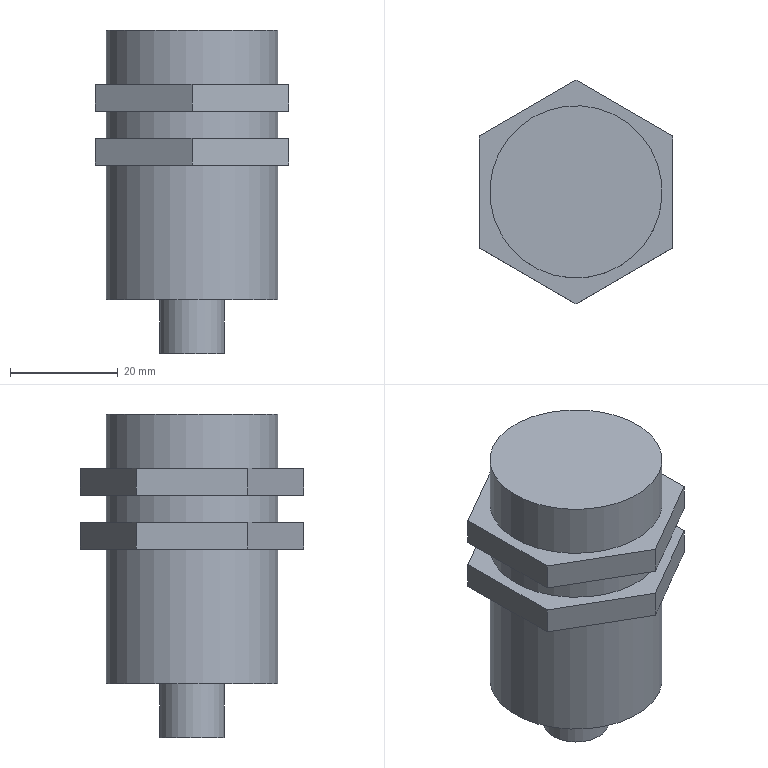Part | NX | features solid 2 | 1 solid | 23 faces | box 36 x 41.569 x 60 mm | volume 44525 mm3 | plane 19 | cylinder 4 | commonest cylinder face diameters 32 x3 12 x1
STEP:
#1=CARTESIAN_POINT('',(1648.644,144.279,-60.));
#2=VERTEX_POINT('',#1);
#3=CARTESIAN_POINT('',(1634.788,136.279,-60.));
#4=DIRECTION('',(0.,0.,-1.));
#5=DIRECTION('',(0.866,0.5,0.));
#6=AXIS2_PLACEMENT_3D('',#3,#4,#5);
#7=CIRCLE('',#6,16.);
#8=EDGE_CURVE('',#2,#2,#7,.T.);
#9=ORIENTED_EDGE('',*,*,#8,.F.);
#10=EDGE_LOOP('',(#9));
#11=FACE_BOUND('',#10,.T.);
#12=CARTESIAN_POINT('',(1648.644,144.279,-55.));
#13=VERTEX_POINT('',#12);
#14=CARTESIAN_POINT('',(1634.788,136.279,-55.));
#15=DIRECTION('',(0.,0.,-1.));
#16=DIRECTION('',(0.866,0.5,0.));
#17=AXIS2_PLACEMENT_3D('',#14,#15,#16);
#18=CIRCLE('',#17,16.);
#19=EDGE_CURVE('',#13,#13,#18,.T.);
#20=ORIENTED_EDGE('',*,*,#19,.T.);
#21=EDGE_LOOP('',(#20));
#22=FACE_BOUND('',#21,.T.);
#23=CARTESIAN_POINT('',(1634.788,136.279,-40.));
#24=DIRECTION('',(0.,0.,-1.));
#25=DIRECTION('',(-0.866,-0.5,0.));
#26=AXIS2_PLACEMENT_3D('',#23,#24,#25);
#27=CYLINDRICAL_SURFACE('',#26,16.);
#28=ADVANCED_FACE('',(#11,#22),#27,.T.);
#29=CARTESIAN_POINT('',(1648.644,144.279,-90.));
#30=VERTEX_POINT('',#29);
#31=CARTESIAN_POINT('',(1634.788,136.279,-90.));
#32=DIRECTION('',(0.,0.,-1.));
#33=DIRECTION('',(0.866,0.5,0.));
#34=AXIS2_PLACEMENT_3D('',#31,#32,#33);
#35=CIRCLE('',#34,16.);
#36=EDGE_CURVE('',#30,#30,#35,.T.);
#37=ORIENTED_EDGE('',*,*,#36,.F.);
#38=EDGE_LOOP('',(#37));
#39=FACE_BOUND('',#38,.T.);
#40=CARTESIAN_POINT('',(1648.644,144.279,-65.));
#41=VERTEX_POINT('',#40);
#42=CARTESIAN_POINT('',(1634.788,136.279,-65.));
#43=DIRECTION('',(0.,0.,-1.));
#44=DIRECTION('',(0.866,0.5,0.));
#45=AXIS2_PLACEMENT_3D('',#42,#43,#44);
#46=CIRCLE('',#45,16.);
#47=EDGE_CURVE('',#41,#41,#46,.T.);
#48=ORIENTED_EDGE('',*,*,#47,.T.);
#49=EDGE_LOOP('',(#48));
#50=FACE_BOUND('',#49,.T.);
#51=CARTESIAN_POINT('',(1634.788,136.279,-40.));
#52=DIRECTION('',(0.,0.,-1.));
#53=DIRECTION('',(-0.866,-0.5,0.));
#54=AXIS2_PLACEMENT_3D('',#51,#52,#53);
#55=CYLINDRICAL_SURFACE('',#54,16.);
#56=ADVANCED_FACE('',(#39,#50),#55,.T.);
#57=CARTESIAN_POINT('',(1639.984,139.279,-90.));
#58=VERTEX_POINT('',#57);
#59=CARTESIAN_POINT('',(1634.788,136.279,-90.));
#60=DIRECTION('',(0.,0.,-1.));
#61=DIRECTION('',(0.866,0.5,0.));
#62=AXIS2_PLACEMENT_3D('',#59,#60,#61);
#63=CIRCLE('',#62,6.);
#64=EDGE_CURVE('',#58,#58,#63,.T.);
#65=ORIENTED_EDGE('',*,*,#64,.T.);
#66=EDGE_LOOP('',(#65));
#67=FACE_BOUND('',#66,.T.);
#68=CARTESIAN_POINT('',(1639.984,139.279,-100.));
#69=VERTEX_POINT('',#68);
#70=CARTESIAN_POINT('',(1634.788,136.279,-100.));
#71=DIRECTION('',(0.,0.,-1.));
#72=DIRECTION('',(0.866,0.5,0.));
#73=AXIS2_PLACEMENT_3D('',#70,#71,#72);
#74=CIRCLE('',#73,6.);
#75=EDGE_CURVE('',#69,#69,#74,.T.);
#76=ORIENTED_EDGE('',*,*,#75,.F.);
#77=EDGE_LOOP('',(#76));
#78=FACE_BOUND('',#77,.T.);
#79=CARTESIAN_POINT('',(1634.788,136.279,-90.));
#80=DIRECTION('',(0.,0.,-1.));
#81=DIRECTION('',(-0.866,-0.5,0.));
#82=AXIS2_PLACEMENT_3D('',#79,#80,#81);
#83=CYLINDRICAL_SURFACE('',#82,6.);
#84=ADVANCED_FACE('',(#67,#78),#83,.T.);
#85=ORIENTED_EDGE('',*,*,#75,.T.);
#86=EDGE_LOOP('',(#85));
#87=FACE_BOUND('',#86,.T.);
#88=CARTESIAN_POINT('',(1634.788,136.279,-100.));
#89=DIRECTION('',(0.,0.,1.));
#90=DIRECTION('',(0.866,0.5,0.));
#91=AXIS2_PLACEMENT_3D('',#88,#89,#90);
#92=PLANE('',#91);
#93=ADVANCED_FACE('',(#87),#92,.F.);
#94=ORIENTED_EDGE('',*,*,#36,.T.);
#95=EDGE_LOOP('',(#94));
#96=FACE_BOUND('',#95,.T.);
#97=ORIENTED_EDGE('',*,*,#64,.F.);
#98=EDGE_LOOP('',(#97));
#99=FACE_BOUND('',#98,.T.);
#100=CARTESIAN_POINT('',(1634.788,136.279,-90.));
#101=DIRECTION('',(0.,0.,1.));
#102=DIRECTION('',(0.866,0.5,0.));
#103=AXIS2_PLACEMENT_3D('',#100,#101,#102);
#104=PLANE('',#103);
#105=ADVANCED_FACE('',(#96,#99),#104,.F.);
#106=CARTESIAN_POINT('',(1616.788,125.887,-60.));
#107=VERTEX_POINT('',#106);
#108=CARTESIAN_POINT('',(1634.788,115.495,-60.));
#109=VERTEX_POINT('',#108);
#110=CARTESIAN_POINT('',(1616.788,125.887,-60.));
#111=DIRECTION('',(0.866,-0.5,0.));
#112=VECTOR('',#111,1000.);
#113=LINE('',#110,#112);
#114=EDGE_CURVE('',#107,#109,#113,.T.);
#115=ORIENTED_EDGE('',*,*,#114,.T.);
#116=CARTESIAN_POINT('',(1652.788,125.887,-60.));
#117=VERTEX_POINT('',#116);
#118=CARTESIAN_POINT('',(1634.788,115.495,-60.));
#119=DIRECTION('',(0.866,0.5,0.));
#120=VECTOR('',#119,1000.);
#121=LINE('',#118,#120);
#122=EDGE_CURVE('',#109,#117,#121,.T.);
#123=ORIENTED_EDGE('',*,*,#122,.T.);
#124=CARTESIAN_POINT('',(1652.788,146.672,-60.));
#125=VERTEX_POINT('',#124);
#126=CARTESIAN_POINT('',(1652.788,146.672,-60.));
#127=DIRECTION('',(0.,-1.,0.));
#128=VECTOR('',#127,1000.);
#129=LINE('',#126,#128);
#130=EDGE_CURVE('',#125,#117,#129,.T.);
#131=ORIENTED_EDGE('',*,*,#130,.F.);
#132=CARTESIAN_POINT('',(1634.788,157.064,-60.));
#133=VERTEX_POINT('',#132);
#134=CARTESIAN_POINT('',(1652.788,146.672,-60.));
#135=DIRECTION('',(-0.866,0.5,0.));
#136=VECTOR('',#135,1000.);
#137=LINE('',#134,#136);
#138=EDGE_CURVE('',#125,#133,#137,.T.);
#139=ORIENTED_EDGE('',*,*,#138,.T.);
#140=CARTESIAN_POINT('',(1616.788,146.672,-60.));
#141=VERTEX_POINT('',#140);
#142=CARTESIAN_POINT('',(1634.788,157.064,-60.));
#143=DIRECTION('',(-0.866,-0.5,0.));
#144=VECTOR('',#143,1000.);
#145=LINE('',#142,#144);
#146=EDGE_CURVE('',#133,#141,#145,.T.);
#147=ORIENTED_EDGE('',*,*,#146,.T.);
#148=CARTESIAN_POINT('',(1616.788,146.672,-60.));
#149=DIRECTION('',(0.,-1.,0.));
#150=VECTOR('',#149,1000.);
#151=LINE('',#148,#150);
#152=EDGE_CURVE('',#141,#107,#151,.T.);
#153=ORIENTED_EDGE('',*,*,#152,.T.);
#154=EDGE_LOOP('',(#115,#123,#131,#139,#147,#153));
#155=FACE_BOUND('',#154,.T.);
#156=ORIENTED_EDGE('',*,*,#8,.T.);
#157=EDGE_LOOP('',(#156));
#158=FACE_BOUND('',#157,.T.);
#159=CARTESIAN_POINT('',(1652.788,105.103,-60.));
#160=DIRECTION('',(0.,0.,1.));
#161=DIRECTION('',(0.866,0.5,0.));
#162=AXIS2_PLACEMENT_3D('',#159,#160,#161);
#163=PLANE('',#162);
#164=ADVANCED_FACE('',(#155,#158),#163,.T.);
#165=CARTESIAN_POINT('',(1616.788,125.887,-65.));
#166=VERTEX_POINT('',#165);
#167=CARTESIAN_POINT('',(1634.788,115.495,-65.));
#168=VERTEX_POINT('',#167);
#169=CARTESIAN_POINT('',(1616.788,125.887,-65.));
#170=DIRECTION('',(0.866,-0.5,0.));
#171=VECTOR('',#170,1000.);
#172=LINE('',#169,#171);
#173=EDGE_CURVE('',#166,#168,#172,.T.);
#174=ORIENTED_EDGE('',*,*,#173,.F.);
#175=CARTESIAN_POINT('',(1616.788,146.672,-65.));
#176=VERTEX_POINT('',#175);
#177=CARTESIAN_POINT('',(1616.788,146.672,-65.));
#178=DIRECTION('',(0.,-1.,0.));
#179=VECTOR('',#178,1000.);
#180=LINE('',#177,#179);
#181=EDGE_CURVE('',#176,#166,#180,.T.);
#182=ORIENTED_EDGE('',*,*,#181,.F.);
#183=CARTESIAN_POINT('',(1634.788,157.064,-65.));
#184=VERTEX_POINT('',#183);
#185=CARTESIAN_POINT('',(1634.788,157.064,-65.));
#186=DIRECTION('',(-0.866,-0.5,0.));
#187=VECTOR('',#186,1000.);
#188=LINE('',#185,#187);
#189=EDGE_CURVE('',#184,#176,#188,.T.);
#190=ORIENTED_EDGE('',*,*,#189,.F.);
#191=CARTESIAN_POINT('',(1652.788,146.672,-65.));
#192=VERTEX_POINT('',#191);
#193=CARTESIAN_POINT('',(1652.788,146.672,-65.));
#194=DIRECTION('',(-0.866,0.5,0.));
#195=VECTOR('',#194,1000.);
#196=LINE('',#193,#195);
#197=EDGE_CURVE('',#192,#184,#196,.T.);
#198=ORIENTED_EDGE('',*,*,#197,.F.);
#199=CARTESIAN_POINT('',(1652.788,125.887,-65.));
#200=VERTEX_POINT('',#199);
#201=CARTESIAN_POINT('',(1652.788,146.672,-65.));
#202=DIRECTION('',(0.,-1.,0.));
#203=VECTOR('',#202,1000.);
#204=LINE('',#201,#203);
#205=EDGE_CURVE('',#192,#200,#204,.T.);
#206=ORIENTED_EDGE('',*,*,#205,.T.);
#207=CARTESIAN_POINT('',(1634.788,115.495,-65.));
#208=DIRECTION('',(0.866,0.5,0.));
#209=VECTOR('',#208,1000.);
#210=LINE('',#207,#209);
#211=EDGE_CURVE('',#168,#200,#210,.T.);
#212=ORIENTED_EDGE('',*,*,#211,.F.);
#213=EDGE_LOOP('',(#174,#182,#190,#198,#206,#212));
#214=FACE_BOUND('',#213,.T.);
#215=ORIENTED_EDGE('',*,*,#47,.F.);
#216=EDGE_LOOP('',(#215));
#217=FACE_BOUND('',#216,.T.);
#218=CARTESIAN_POINT('',(1652.788,105.103,-65.));
#219=DIRECTION('',(0.,0.,1.));
#220=DIRECTION('',(0.866,0.5,0.));
#221=AXIS2_PLACEMENT_3D('',#218,#219,#220);
#222=PLANE('',#221);
#223=ADVANCED_FACE('',(#214,#217),#222,.F.);
#224=ORIENTED_EDGE('',*,*,#173,.T.);
#225=CARTESIAN_POINT('',(1634.788,115.495,-60.));
#226=DIRECTION('',(0.,0.,-1.));
#227=VECTOR('',#226,1000.);
#228=LINE('',#225,#227);
#229=EDGE_CURVE('',#109,#168,#228,.T.);
#230=ORIENTED_EDGE('',*,*,#229,.F.);
#231=ORIENTED_EDGE('',*,*,#114,.F.);
#232=CARTESIAN_POINT('',(1616.788,125.887,-60.));
#233=DIRECTION('',(0.,0.,-1.));
#234=VECTOR('',#233,1000.);
#235=LINE('',#232,#234);
#236=EDGE_CURVE('',#107,#166,#235,.T.);
#237=ORIENTED_EDGE('',*,*,#236,.T.);
#238=EDGE_LOOP('',(#224,#230,#231,#237));
#239=FACE_BOUND('',#238,.T.);
#240=CARTESIAN_POINT('',(1616.788,125.887,-60.));
#241=DIRECTION('',(-0.5,-0.866,0.));
#242=DIRECTION('',(-0.866,0.5,0.));
#243=AXIS2_PLACEMENT_3D('',#240,#241,#242);
#244=PLANE('',#243);
#245=ADVANCED_FACE('',(#239),#244,.T.);
#246=ORIENTED_EDGE('',*,*,#211,.T.);
#247=CARTESIAN_POINT('',(1652.788,125.887,-60.));
#248=DIRECTION('',(0.,0.,-1.));
#249=VECTOR('',#248,1000.);
#250=LINE('',#247,#249);
#251=EDGE_CURVE('',#117,#200,#250,.T.);
#252=ORIENTED_EDGE('',*,*,#251,.F.);
#253=ORIENTED_EDGE('',*,*,#122,.F.);
#254=ORIENTED_EDGE('',*,*,#229,.T.);
#255=EDGE_LOOP('',(#246,#252,#253,#254));
#256=FACE_BOUND('',#255,.T.);
#257=CARTESIAN_POINT('',(1634.788,115.495,-60.));
#258=DIRECTION('',(0.5,-0.866,0.));
#259=DIRECTION('',(0.,0.,1.));
#260=AXIS2_PLACEMENT_3D('',#257,#258,#259);
#261=PLANE('',#260);
#262=ADVANCED_FACE('',(#256),#261,.T.);
#263=ORIENTED_EDGE('',*,*,#205,.F.);
#264=CARTESIAN_POINT('',(1652.788,146.672,-60.));
#265=DIRECTION('',(0.,0.,-1.));
#266=VECTOR('',#265,1000.);
#267=LINE('',#264,#266);
#268=EDGE_CURVE('',#125,#192,#267,.T.);
#269=ORIENTED_EDGE('',*,*,#268,.F.);
#270=ORIENTED_EDGE('',*,*,#130,.T.);
#271=ORIENTED_EDGE('',*,*,#251,.T.);
#272=EDGE_LOOP('',(#263,#269,#270,#271));
#273=FACE_BOUND('',#272,.T.);
#274=CARTESIAN_POINT('',(1652.788,146.672,-60.));
#275=DIRECTION('',(-1.,0.,0.));
#276=DIRECTION('',(0.,1.,0.));
#277=AXIS2_PLACEMENT_3D('',#274,#275,#276);
#278=PLANE('',#277);
#279=ADVANCED_FACE('',(#273),#278,.F.);
#280=ORIENTED_EDGE('',*,*,#197,.T.);
#281=CARTESIAN_POINT('',(1634.788,157.064,-60.));
#282=DIRECTION('',(0.,0.,-1.));
#283=VECTOR('',#282,1000.);
#284=LINE('',#281,#283);
#285=EDGE_CURVE('',#133,#184,#284,.T.);
#286=ORIENTED_EDGE('',*,*,#285,.F.);
#287=ORIENTED_EDGE('',*,*,#138,.F.);
#288=ORIENTED_EDGE('',*,*,#268,.T.);
#289=EDGE_LOOP('',(#280,#286,#287,#288));
#290=FACE_BOUND('',#289,.T.);
#291=CARTESIAN_POINT('',(1652.788,146.672,-60.));
#292=DIRECTION('',(0.5,0.866,0.));
#293=DIRECTION('',(0.866,-0.5,0.));
#294=AXIS2_PLACEMENT_3D('',#291,#292,#293);
#295=PLANE('',#294);
#296=ADVANCED_FACE('',(#290),#295,.T.);
#297=ORIENTED_EDGE('',*,*,#189,.T.);
#298=CARTESIAN_POINT('',(1616.788,146.672,-60.));
#299=DIRECTION('',(0.,0.,-1.));
#300=VECTOR('',#299,1000.);
#301=LINE('',#298,#300);
#302=EDGE_CURVE('',#141,#176,#301,.T.);
#303=ORIENTED_EDGE('',*,*,#302,.F.);
#304=ORIENTED_EDGE('',*,*,#146,.F.);
#305=ORIENTED_EDGE('',*,*,#285,.T.);
#306=EDGE_LOOP('',(#297,#303,#304,#305));
#307=FACE_BOUND('',#306,.T.);
#308=CARTESIAN_POINT('',(1634.788,157.064,-60.));
#309=DIRECTION('',(-0.5,0.866,0.));
#310=DIRECTION('',(0.866,0.5,0.));
#311=AXIS2_PLACEMENT_3D('',#308,#309,#310);
#312=PLANE('',#311);
#313=ADVANCED_FACE('',(#307),#312,.T.);
#314=ORIENTED_EDGE('',*,*,#181,.T.);
#315=ORIENTED_EDGE('',*,*,#236,.F.);
#316=ORIENTED_EDGE('',*,*,#152,.F.);
#317=ORIENTED_EDGE('',*,*,#302,.T.);
#318=EDGE_LOOP('',(#314,#315,#316,#317));
#319=FACE_BOUND('',#318,.T.);
#320=CARTESIAN_POINT('',(1616.788,146.672,-60.));
#321=DIRECTION('',(-1.,0.,0.));
#322=DIRECTION('',(0.,1.,0.));
#323=AXIS2_PLACEMENT_3D('',#320,#321,#322);
#324=PLANE('',#323);
#325=ADVANCED_FACE('',(#319),#324,.T.);
#326=CARTESIAN_POINT('',(1616.788,146.672,-50.));
#327=VERTEX_POINT('',#326);
#328=CARTESIAN_POINT('',(1616.788,125.887,-50.));
#329=VERTEX_POINT('',#328);
#330=CARTESIAN_POINT('',(1616.788,146.672,-50.));
#331=DIRECTION('',(0.,-1.,0.));
#332=VECTOR('',#331,1000.);
#333=LINE('',#330,#332);
#334=EDGE_CURVE('',#327,#329,#333,.T.);
#335=ORIENTED_EDGE('',*,*,#334,.T.);
#336=CARTESIAN_POINT('',(1634.788,115.495,-50.));
#337=VERTEX_POINT('',#336);
#338=CARTESIAN_POINT('',(1616.788,125.887,-50.));
#339=DIRECTION('',(0.866,-0.5,0.));
#340=VECTOR('',#339,1000.);
#341=LINE('',#338,#340);
#342=EDGE_CURVE('',#329,#337,#341,.T.);
#343=ORIENTED_EDGE('',*,*,#342,.T.);
#344=CARTESIAN_POINT('',(1652.788,125.887,-50.));
#345=VERTEX_POINT('',#344);
#346=CARTESIAN_POINT('',(1634.788,115.495,-50.));
#347=DIRECTION('',(0.866,0.5,0.));
#348=VECTOR('',#347,1000.);
#349=LINE('',#346,#348);
#350=EDGE_CURVE('',#337,#345,#349,.T.);
#351=ORIENTED_EDGE('',*,*,#350,.T.);
#352=CARTESIAN_POINT('',(1652.788,146.672,-50.));
#353=VERTEX_POINT('',#352);
#354=CARTESIAN_POINT('',(1652.788,146.672,-50.));
#355=DIRECTION('',(0.,-1.,0.));
#356=VECTOR('',#355,1000.);
#357=LINE('',#354,#356);
#358=EDGE_CURVE('',#353,#345,#357,.T.);
#359=ORIENTED_EDGE('',*,*,#358,.F.);
#360=CARTESIAN_POINT('',(1634.788,157.064,-50.));
#361=VERTEX_POINT('',#360);
#362=CARTESIAN_POINT('',(1652.788,146.672,-50.));
#363=DIRECTION('',(-0.866,0.5,0.));
#364=VECTOR('',#363,1000.);
#365=LINE('',#362,#364);
#366=EDGE_CURVE('',#353,#361,#365,.T.);
#367=ORIENTED_EDGE('',*,*,#366,.T.);
#368=CARTESIAN_POINT('',(1634.788,157.064,-50.));
#369=DIRECTION('',(-0.866,-0.5,0.));
#370=VECTOR('',#369,1000.);
#371=LINE('',#368,#370);
#372=EDGE_CURVE('',#361,#327,#371,.T.);
#373=ORIENTED_EDGE('',*,*,#372,.T.);
#374=EDGE_LOOP('',(#335,#343,#351,#359,#367,#373));
#375=FACE_BOUND('',#374,.T.);
#376=CARTESIAN_POINT('',(1648.644,144.279,-50.));
#377=VERTEX_POINT('',#376);
#378=CARTESIAN_POINT('',(1634.788,136.279,-50.));
#379=DIRECTION('',(0.,0.,-1.));
#380=DIRECTION('',(0.866,0.5,0.));
#381=AXIS2_PLACEMENT_3D('',#378,#379,#380);
#382=CIRCLE('',#381,16.);
#383=EDGE_CURVE('',#377,#377,#382,.T.);
#384=ORIENTED_EDGE('',*,*,#383,.T.);
#385=EDGE_LOOP('',(#384));
#386=FACE_BOUND('',#385,.T.);
#387=CARTESIAN_POINT('',(1616.788,167.456,-50.));
#388=DIRECTION('',(0.,0.,1.));
#389=DIRECTION('',(0.866,0.5,0.));
#390=AXIS2_PLACEMENT_3D('',#387,#388,#389);
#391=PLANE('',#390);
#392=ADVANCED_FACE('',(#375,#386),#391,.T.);
#393=CARTESIAN_POINT('',(1616.788,146.672,-55.));
#394=VERTEX_POINT('',#393);
#395=CARTESIAN_POINT('',(1616.788,125.887,-55.));
#396=VERTEX_POINT('',#395);
#397=CARTESIAN_POINT('',(1616.788,146.672,-55.));
#398=DIRECTION('',(0.,-1.,0.));
#399=VECTOR('',#398,1000.);
#400=LINE('',#397,#399);
#401=EDGE_CURVE('',#394,#396,#400,.T.);
#402=ORIENTED_EDGE('',*,*,#401,.F.);
#403=CARTESIAN_POINT('',(1634.788,157.064,-55.));
#404=VERTEX_POINT('',#403);
#405=CARTESIAN_POINT('',(1634.788,157.064,-55.));
#406=DIRECTION('',(-0.866,-0.5,0.));
#407=VECTOR('',#406,1000.);
#408=LINE('',#405,#407);
#409=EDGE_CURVE('',#404,#394,#408,.T.);
#410=ORIENTED_EDGE('',*,*,#409,.F.);
#411=CARTESIAN_POINT('',(1652.788,146.672,-55.));
#412=VERTEX_POINT('',#411);
#413=CARTESIAN_POINT('',(1652.788,146.672,-55.));
#414=DIRECTION('',(-0.866,0.5,0.));
#415=VECTOR('',#414,1000.);
#416=LINE('',#413,#415);
#417=EDGE_CURVE('',#412,#404,#416,.T.);
#418=ORIENTED_EDGE('',*,*,#417,.F.);
#419=CARTESIAN_POINT('',(1652.788,125.887,-55.));
#420=VERTEX_POINT('',#419);
#421=CARTESIAN_POINT('',(1652.788,146.672,-55.));
#422=DIRECTION('',(0.,-1.,0.));
#423=VECTOR('',#422,1000.);
#424=LINE('',#421,#423);
#425=EDGE_CURVE('',#412,#420,#424,.T.);
#426=ORIENTED_EDGE('',*,*,#425,.T.);
#427=CARTESIAN_POINT('',(1634.788,115.495,-55.));
#428=VERTEX_POINT('',#427);
#429=CARTESIAN_POINT('',(1634.788,115.495,-55.));
#430=DIRECTION('',(0.866,0.5,0.));
#431=VECTOR('',#430,1000.);
#432=LINE('',#429,#431);
#433=EDGE_CURVE('',#428,#420,#432,.T.);
#434=ORIENTED_EDGE('',*,*,#433,.F.);
#435=CARTESIAN_POINT('',(1616.788,125.887,-55.));
#436=DIRECTION('',(0.866,-0.5,0.));
#437=VECTOR('',#436,1000.);
#438=LINE('',#435,#437);
#439=EDGE_CURVE('',#396,#428,#438,.T.);
#440=ORIENTED_EDGE('',*,*,#439,.F.);
#441=EDGE_LOOP('',(#402,#410,#418,#426,#434,#440));
#442=FACE_BOUND('',#441,.T.);
#443=ORIENTED_EDGE('',*,*,#19,.F.);
#444=EDGE_LOOP('',(#443));
#445=FACE_BOUND('',#444,.T.);
#446=CARTESIAN_POINT('',(1616.788,167.456,-55.));
#447=DIRECTION('',(0.,0.,1.));
#448=DIRECTION('',(0.866,0.5,0.));
#449=AXIS2_PLACEMENT_3D('',#446,#447,#448);
#450=PLANE('',#449);
#451=ADVANCED_FACE('',(#442,#445),#450,.F.);
#452=ORIENTED_EDGE('',*,*,#401,.T.);
#453=CARTESIAN_POINT('',(1616.788,125.887,-50.));
#454=DIRECTION('',(0.,0.,-1.));
#455=VECTOR('',#454,1000.);
#456=LINE('',#453,#455);
#457=EDGE_CURVE('',#329,#396,#456,.T.);
#458=ORIENTED_EDGE('',*,*,#457,.F.);
#459=ORIENTED_EDGE('',*,*,#334,.F.);
#460=CARTESIAN_POINT('',(1616.788,146.672,-50.));
#461=DIRECTION('',(0.,0.,-1.));
#462=VECTOR('',#461,1000.);
#463=LINE('',#460,#462);
#464=EDGE_CURVE('',#327,#394,#463,.T.);
#465=ORIENTED_EDGE('',*,*,#464,.T.);
#466=EDGE_LOOP('',(#452,#458,#459,#465));
#467=FACE_BOUND('',#466,.T.);
#468=CARTESIAN_POINT('',(1616.788,146.672,-50.));
#469=DIRECTION('',(-1.,0.,0.));
#470=DIRECTION('',(0.,1.,0.));
#471=AXIS2_PLACEMENT_3D('',#468,#469,#470);
#472=PLANE('',#471);
#473=ADVANCED_FACE('',(#467),#472,.T.);
#474=ORIENTED_EDGE('',*,*,#439,.T.);
#475=CARTESIAN_POINT('',(1634.788,115.495,-50.));
#476=DIRECTION('',(0.,0.,-1.));
#477=VECTOR('',#476,1000.);
#478=LINE('',#475,#477);
#479=EDGE_CURVE('',#337,#428,#478,.T.);
#480=ORIENTED_EDGE('',*,*,#479,.F.);
#481=ORIENTED_EDGE('',*,*,#342,.F.);
#482=ORIENTED_EDGE('',*,*,#457,.T.);
#483=EDGE_LOOP('',(#474,#480,#481,#482));
#484=FACE_BOUND('',#483,.T.);
#485=CARTESIAN_POINT('',(1616.788,125.887,-50.));
#486=DIRECTION('',(-0.5,-0.866,0.));
#487=DIRECTION('',(-0.866,0.5,0.));
#488=AXIS2_PLACEMENT_3D('',#485,#486,#487);
#489=PLANE('',#488);
#490=ADVANCED_FACE('',(#484),#489,.T.);
#491=ORIENTED_EDGE('',*,*,#433,.T.);
#492=CARTESIAN_POINT('',(1652.788,125.887,-50.));
#493=DIRECTION('',(0.,0.,-1.));
#494=VECTOR('',#493,1000.);
#495=LINE('',#492,#494);
#496=EDGE_CURVE('',#345,#420,#495,.T.);
#497=ORIENTED_EDGE('',*,*,#496,.F.);
#498=ORIENTED_EDGE('',*,*,#350,.F.);
#499=ORIENTED_EDGE('',*,*,#479,.T.);
#500=EDGE_LOOP('',(#491,#497,#498,#499));
#501=FACE_BOUND('',#500,.T.);
#502=CARTESIAN_POINT('',(1634.788,115.495,-50.));
#503=DIRECTION('',(0.5,-0.866,0.));
#504=DIRECTION('',(0.,0.,1.));
#505=AXIS2_PLACEMENT_3D('',#502,#503,#504);
#506=PLANE('',#505);
#507=ADVANCED_FACE('',(#501),#506,.T.);
#508=ORIENTED_EDGE('',*,*,#425,.F.);
#509=CARTESIAN_POINT('',(1652.788,146.672,-50.));
#510=DIRECTION('',(0.,0.,-1.));
#511=VECTOR('',#510,1000.);
#512=LINE('',#509,#511);
#513=EDGE_CURVE('',#353,#412,#512,.T.);
#514=ORIENTED_EDGE('',*,*,#513,.F.);
#515=ORIENTED_EDGE('',*,*,#358,.T.);
#516=ORIENTED_EDGE('',*,*,#496,.T.);
#517=EDGE_LOOP('',(#508,#514,#515,#516));
#518=FACE_BOUND('',#517,.T.);
#519=CARTESIAN_POINT('',(1652.788,146.672,-50.));
#520=DIRECTION('',(-1.,0.,0.));
#521=DIRECTION('',(0.,1.,0.));
#522=AXIS2_PLACEMENT_3D('',#519,#520,#521);
#523=PLANE('',#522);
#524=ADVANCED_FACE('',(#518),#523,.F.);
#525=ORIENTED_EDGE('',*,*,#417,.T.);
#526=CARTESIAN_POINT('',(1634.788,157.064,-50.));
#527=DIRECTION('',(0.,0.,-1.));
#528=VECTOR('',#527,1000.);
#529=LINE('',#526,#528);
#530=EDGE_CURVE('',#361,#404,#529,.T.);
#531=ORIENTED_EDGE('',*,*,#530,.F.);
#532=ORIENTED_EDGE('',*,*,#366,.F.);
#533=ORIENTED_EDGE('',*,*,#513,.T.);
#534=EDGE_LOOP('',(#525,#531,#532,#533));
#535=FACE_BOUND('',#534,.T.);
#536=CARTESIAN_POINT('',(1652.788,146.672,-50.));
#537=DIRECTION('',(0.5,0.866,0.));
#538=DIRECTION('',(0.866,-0.5,0.));
#539=AXIS2_PLACEMENT_3D('',#536,#537,#538);
#540=PLANE('',#539);
#541=ADVANCED_FACE('',(#535),#540,.T.);
#542=ORIENTED_EDGE('',*,*,#409,.T.);
#543=ORIENTED_EDGE('',*,*,#464,.F.);
#544=ORIENTED_EDGE('',*,*,#372,.F.);
#545=ORIENTED_EDGE('',*,*,#530,.T.);
#546=EDGE_LOOP('',(#542,#543,#544,#545));
#547=FACE_BOUND('',#546,.T.);
#548=CARTESIAN_POINT('',(1634.788,157.064,-50.));
#549=DIRECTION('',(-0.5,0.866,0.));
#550=DIRECTION('',(0.866,0.5,0.));
#551=AXIS2_PLACEMENT_3D('',#548,#549,#550);
#552=PLANE('',#551);
#553=ADVANCED_FACE('',(#547),#552,.T.);
#554=CARTESIAN_POINT('',(1648.644,144.279,-40.));
#555=VERTEX_POINT('',#554);
#556=CARTESIAN_POINT('',(1634.788,136.279,-40.));
#557=DIRECTION('',(0.,0.,-1.));
#558=DIRECTION('',(0.866,0.5,0.));
#559=AXIS2_PLACEMENT_3D('',#556,#557,#558);
#560=CIRCLE('',#559,16.);
#561=EDGE_CURVE('',#555,#555,#560,.T.);
#562=ORIENTED_EDGE('',*,*,#561,.F.);
#563=EDGE_LOOP('',(#562));
#564=FACE_BOUND('',#563,.T.);
#565=CARTESIAN_POINT('',(1634.788,136.279,-40.));
#566=DIRECTION('',(0.,0.,1.));
#567=DIRECTION('',(0.866,0.5,0.));
#568=AXIS2_PLACEMENT_3D('',#565,#566,#567);
#569=PLANE('',#568);
#570=ADVANCED_FACE('',(#564),#569,.T.);
#571=ORIENTED_EDGE('',*,*,#383,.F.);
#572=EDGE_LOOP('',(#571));
#573=FACE_BOUND('',#572,.T.);
#574=ORIENTED_EDGE('',*,*,#561,.T.);
#575=EDGE_LOOP('',(#574));
#576=FACE_BOUND('',#575,.T.);
#577=CARTESIAN_POINT('',(1634.788,136.279,-40.));
#578=DIRECTION('',(0.,0.,-1.));
#579=DIRECTION('',(-0.866,-0.5,0.));
#580=AXIS2_PLACEMENT_3D('',#577,#578,#579);
#581=CYLINDRICAL_SURFACE('',#580,16.);
#582=ADVANCED_FACE('',(#573,#576),#581,.T.);
#583=CLOSED_SHELL('',(#28,#56,#84,#93,#105,#164,#223,#245,#262,#279,#296,#313,#325,#392,#451,#473,#490,#507,#524,#541,#553,#570,#582));
#584=MANIFOLD_SOLID_BREP('',#583);
#585=(LENGTH_UNIT()NAMED_UNIT(*)SI_UNIT(.MILLI.,.METRE.));
#586=UNCERTAINTY_MEASURE_WITH_UNIT(LENGTH_MEASURE(0.00001),#585,'','');
#587=(NAMED_UNIT(*)PLANE_ANGLE_UNIT()SI_UNIT($,.RADIAN.));
#588=(NAMED_UNIT(*)SI_UNIT($,.STERADIAN.)SOLID_ANGLE_UNIT());
#589=(GEOMETRIC_REPRESENTATION_CONTEXT(3)GLOBAL_UNCERTAINTY_ASSIGNED_CONTEXT((#586))GLOBAL_UNIT_ASSIGNED_CONTEXT((#585,#587,#588))REPRESENTATION_CONTEXT('',''));
#590=ADVANCED_BREP_SHAPE_REPRESENTATION('',(#584),#589);